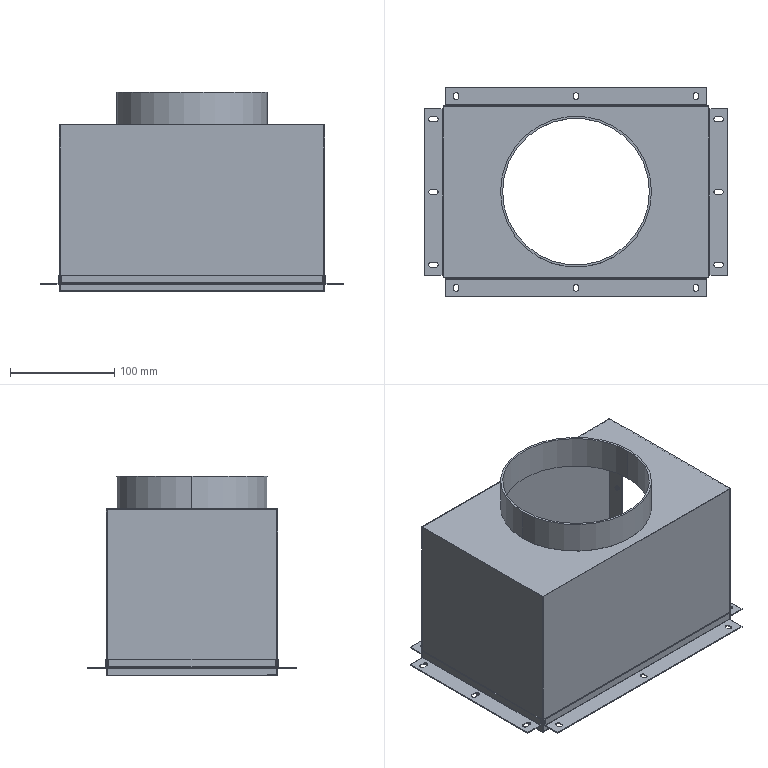Part | STEP file | RJWD-DY-0115-0002 | 14 solids | 215 faces | box 291 x 201 x 191.2 mm | volume 195011 mm3 | plane 118 | cylinder 97 | commonest cylinder face diameters 3 x32 5 x24 4.2 x16 0.4 x5 2 x5 2.4 x5